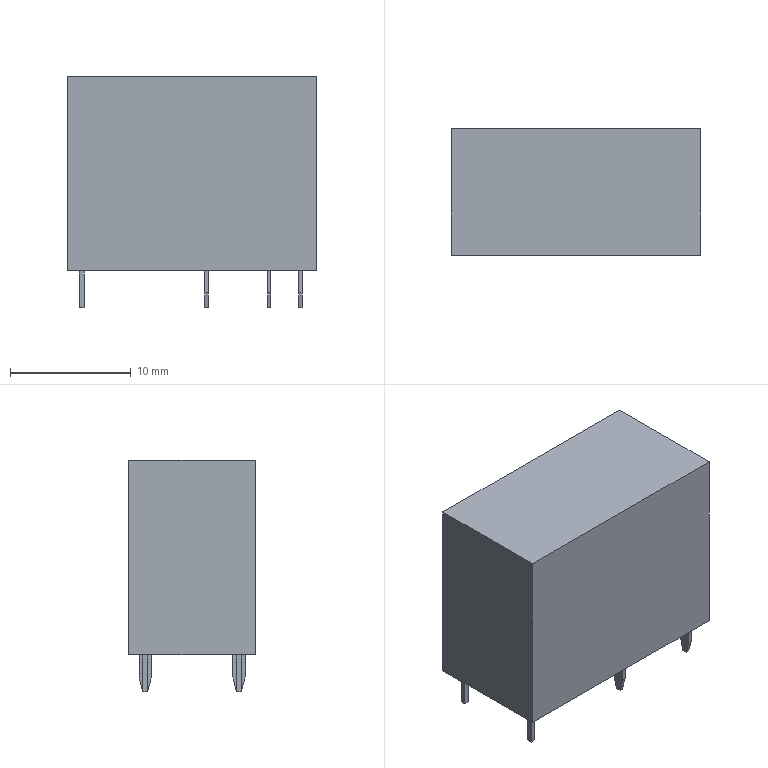Part | NX | features BREP 6 | 6 solids | 330 faces | box 20.662 x 10.494 x 19.135 mm | volume 3407 mm3 | plane 218 | spline 112